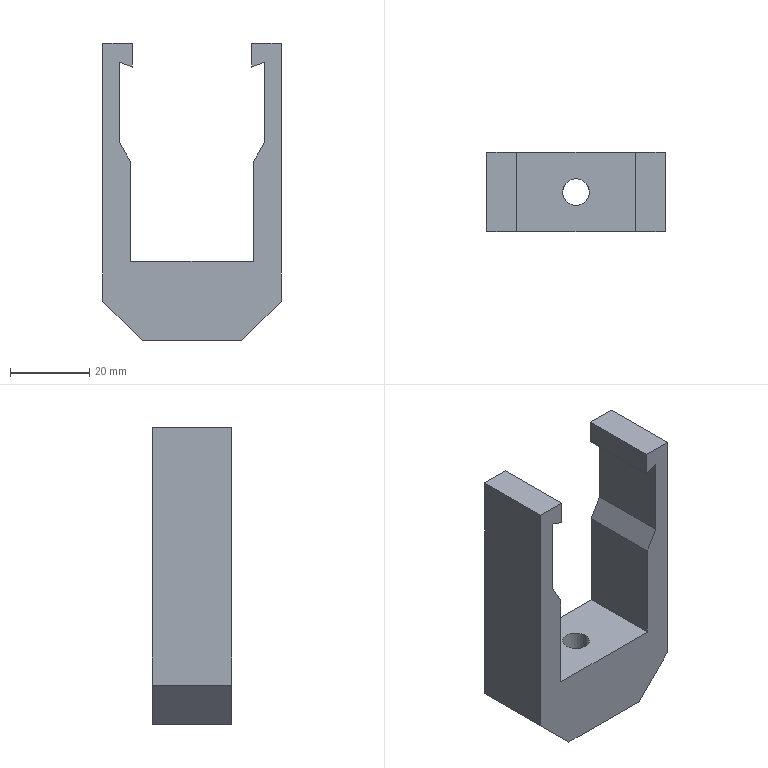Part | STEP file | Blade holder 1 | 1 solid | 22 faces | box 45 x 20 x 75 mm | volume 28350 mm3 | plane 20 | cylinder 2 | commonest cylinder face diameters 6.75 x2
STEP:
#1=CARTESIAN_POINT('',(-3.375,7.5,-37.5));
#2=VERTEX_POINT('',#1);
#3=CARTESIAN_POINT('',(3.375,7.5,-37.5));
#4=VERTEX_POINT('',#3);
#5=CARTESIAN_POINT('',(0.,7.5,-37.5));
#6=DIRECTION('',(0.,0.,1.));
#7=DIRECTION('',(1.,0.,0.));
#8=AXIS2_PLACEMENT_3D('',#5,#6,#7);
#9=CIRCLE('',#8,3.375);
#10=EDGE_CURVE('',#2,#4,#9,.T.);
#11=ORIENTED_EDGE('',*,*,#10,.F.);
#12=CARTESIAN_POINT('',(-3.375,7.5,-17.5));
#13=VERTEX_POINT('',#12);
#14=CARTESIAN_POINT('',(-3.375,7.5,-17.5));
#15=DIRECTION('',(0.,0.,1.));
#16=VECTOR('',#15,1000.);
#17=LINE('',#14,#16);
#18=EDGE_CURVE('',#2,#13,#17,.T.);
#19=ORIENTED_EDGE('',*,*,#18,.T.);
#20=CARTESIAN_POINT('',(3.375,7.5,-17.5));
#21=VERTEX_POINT('',#20);
#22=CARTESIAN_POINT('',(0.,7.5,-17.5));
#23=DIRECTION('',(0.,0.,1.));
#24=DIRECTION('',(1.,0.,0.));
#25=AXIS2_PLACEMENT_3D('',#22,#23,#24);
#26=CIRCLE('',#25,3.375);
#27=EDGE_CURVE('',#13,#21,#26,.T.);
#28=ORIENTED_EDGE('',*,*,#27,.T.);
#29=CARTESIAN_POINT('',(3.375,7.5,-17.5));
#30=DIRECTION('',(0.,0.,1.));
#31=VECTOR('',#30,1000.);
#32=LINE('',#29,#31);
#33=EDGE_CURVE('',#4,#21,#32,.T.);
#34=ORIENTED_EDGE('',*,*,#33,.F.);
#35=EDGE_LOOP('',(#11,#19,#28,#34));
#36=FACE_OUTER_BOUND('',#35,.T.);
#37=CARTESIAN_POINT('',(0.,7.5,-17.5));
#38=DIRECTION('',(0.,0.,1.));
#39=DIRECTION('',(1.,0.,0.));
#40=AXIS2_PLACEMENT_3D('',#37,#38,#39);
#41=CYLINDRICAL_SURFACE('',#40,3.375);
#42=ADVANCED_FACE('',(#36),#41,.F.);
#43=CARTESIAN_POINT('',(15.,17.5,37.5));
#44=VERTEX_POINT('',#43);
#45=CARTESIAN_POINT('',(15.,-2.5,37.5));
#46=VERTEX_POINT('',#45);
#47=CARTESIAN_POINT('',(15.,17.5,37.5));
#48=DIRECTION('',(0.,-1.,0.));
#49=VECTOR('',#48,1000.);
#50=LINE('',#47,#49);
#51=EDGE_CURVE('',#44,#46,#50,.T.);
#52=ORIENTED_EDGE('',*,*,#51,.T.);
#53=CARTESIAN_POINT('',(22.5,-2.5,37.5));
#54=VERTEX_POINT('',#53);
#55=CARTESIAN_POINT('',(-22.5,-2.5,37.5));
#56=DIRECTION('',(1.,0.,0.));
#57=VECTOR('',#56,1000.);
#58=LINE('',#55,#57);
#59=EDGE_CURVE('',#46,#54,#58,.T.);
#60=ORIENTED_EDGE('',*,*,#59,.T.);
#61=CARTESIAN_POINT('',(22.5,17.5,37.5));
#62=VERTEX_POINT('',#61);
#63=CARTESIAN_POINT('',(22.5,-2.5,37.5));
#64=DIRECTION('',(0.,1.,0.));
#65=VECTOR('',#64,1000.);
#66=LINE('',#63,#65);
#67=EDGE_CURVE('',#54,#62,#66,.T.);
#68=ORIENTED_EDGE('',*,*,#67,.T.);
#69=CARTESIAN_POINT('',(-22.5,17.5,37.5));
#70=DIRECTION('',(1.,0.,0.));
#71=VECTOR('',#70,1000.);
#72=LINE('',#69,#71);
#73=EDGE_CURVE('',#44,#62,#72,.T.);
#74=ORIENTED_EDGE('',*,*,#73,.F.);
#75=EDGE_LOOP('',(#52,#60,#68,#74));
#76=FACE_OUTER_BOUND('',#75,.T.);
#77=CARTESIAN_POINT('',(-22.5,-2.5,37.5));
#78=DIRECTION('',(0.,0.,1.));
#79=DIRECTION('',(1.,0.,0.));
#80=AXIS2_PLACEMENT_3D('',#77,#78,#79);
#81=PLANE('',#80);
#82=ADVANCED_FACE('',(#76),#81,.T.);
#83=CARTESIAN_POINT('',(22.5,-2.5,-27.5));
#84=VERTEX_POINT('',#83);
#85=CARTESIAN_POINT('',(22.5,-2.5,37.5));
#86=DIRECTION('',(0.,0.,-1.));
#87=VECTOR('',#86,1000.);
#88=LINE('',#85,#87);
#89=EDGE_CURVE('',#54,#84,#88,.T.);
#90=ORIENTED_EDGE('',*,*,#89,.T.);
#91=CARTESIAN_POINT('',(22.5,17.5,-27.5));
#92=VERTEX_POINT('',#91);
#93=CARTESIAN_POINT('',(22.5,-2.5,-27.5));
#94=DIRECTION('',(0.,1.,0.));
#95=VECTOR('',#94,1000.);
#96=LINE('',#93,#95);
#97=EDGE_CURVE('',#84,#92,#96,.T.);
#98=ORIENTED_EDGE('',*,*,#97,.T.);
#99=CARTESIAN_POINT('',(22.5,17.5,37.5));
#100=DIRECTION('',(0.,0.,-1.));
#101=VECTOR('',#100,1000.);
#102=LINE('',#99,#101);
#103=EDGE_CURVE('',#62,#92,#102,.T.);
#104=ORIENTED_EDGE('',*,*,#103,.F.);
#105=ORIENTED_EDGE('',*,*,#67,.F.);
#106=EDGE_LOOP('',(#90,#98,#104,#105));
#107=FACE_OUTER_BOUND('',#106,.T.);
#108=CARTESIAN_POINT('',(22.5,-2.5,37.5));
#109=DIRECTION('',(1.,0.,0.));
#110=DIRECTION('',(0.,0.,-1.));
#111=AXIS2_PLACEMENT_3D('',#108,#109,#110);
#112=PLANE('',#111);
#113=ADVANCED_FACE('',(#107),#112,.T.);
#114=CARTESIAN_POINT('',(-15.,17.5,37.5));
#115=VERTEX_POINT('',#114);
#116=CARTESIAN_POINT('',(-15.,-2.5,37.5));
#117=VERTEX_POINT('',#116);
#118=CARTESIAN_POINT('',(-15.,17.5,37.5));
#119=DIRECTION('',(0.,-1.,0.));
#120=VECTOR('',#119,1000.);
#121=LINE('',#118,#120);
#122=EDGE_CURVE('',#115,#117,#121,.T.);
#123=ORIENTED_EDGE('',*,*,#122,.F.);
#124=CARTESIAN_POINT('',(-22.5,17.5,37.5));
#125=VERTEX_POINT('',#124);
#126=CARTESIAN_POINT('',(-22.5,17.5,37.5));
#127=DIRECTION('',(1.,0.,0.));
#128=VECTOR('',#127,1000.);
#129=LINE('',#126,#128);
#130=EDGE_CURVE('',#125,#115,#129,.T.);
#131=ORIENTED_EDGE('',*,*,#130,.F.);
#132=CARTESIAN_POINT('',(-22.5,-2.5,37.5));
#133=VERTEX_POINT('',#132);
#134=CARTESIAN_POINT('',(-22.5,-2.5,37.5));
#135=DIRECTION('',(0.,1.,0.));
#136=VECTOR('',#135,1000.);
#137=LINE('',#134,#136);
#138=EDGE_CURVE('',#133,#125,#137,.T.);
#139=ORIENTED_EDGE('',*,*,#138,.F.);
#140=CARTESIAN_POINT('',(-22.5,-2.5,37.5));
#141=DIRECTION('',(1.,0.,0.));
#142=VECTOR('',#141,1000.);
#143=LINE('',#140,#142);
#144=EDGE_CURVE('',#133,#117,#143,.T.);
#145=ORIENTED_EDGE('',*,*,#144,.T.);
#146=EDGE_LOOP('',(#123,#131,#139,#145));
#147=FACE_OUTER_BOUND('',#146,.T.);
#148=CARTESIAN_POINT('',(-22.5,-2.5,37.5));
#149=DIRECTION('',(0.,0.,1.));
#150=DIRECTION('',(1.,0.,0.));
#151=AXIS2_PLACEMENT_3D('',#148,#149,#150);
#152=PLANE('',#151);
#153=ADVANCED_FACE('',(#147),#152,.T.);
#154=CARTESIAN_POINT('',(-22.5,17.5,-27.5));
#155=VERTEX_POINT('',#154);
#156=CARTESIAN_POINT('',(-22.5,17.5,-37.5));
#157=DIRECTION('',(0.,0.,1.));
#158=VECTOR('',#157,1000.);
#159=LINE('',#156,#158);
#160=EDGE_CURVE('',#155,#125,#159,.T.);
#161=ORIENTED_EDGE('',*,*,#160,.F.);
#162=CARTESIAN_POINT('',(-22.5,-2.5,-27.5));
#163=VERTEX_POINT('',#162);
#164=CARTESIAN_POINT('',(-22.5,-2.5,-27.5));
#165=DIRECTION('',(0.,-1.,0.));
#166=VECTOR('',#165,1000.);
#167=LINE('',#164,#166);
#168=EDGE_CURVE('',#155,#163,#167,.T.);
#169=ORIENTED_EDGE('',*,*,#168,.T.);
#170=CARTESIAN_POINT('',(-22.5,-2.5,-37.5));
#171=DIRECTION('',(0.,0.,1.));
#172=VECTOR('',#171,1000.);
#173=LINE('',#170,#172);
#174=EDGE_CURVE('',#163,#133,#173,.T.);
#175=ORIENTED_EDGE('',*,*,#174,.T.);
#176=ORIENTED_EDGE('',*,*,#138,.T.);
#177=EDGE_LOOP('',(#161,#169,#175,#176));
#178=FACE_OUTER_BOUND('',#177,.T.);
#179=CARTESIAN_POINT('',(-22.5,-2.5,-37.5));
#180=DIRECTION('',(-1.,0.,0.));
#181=DIRECTION('',(0.,0.,1.));
#182=AXIS2_PLACEMENT_3D('',#179,#180,#181);
#183=PLANE('',#182);
#184=ADVANCED_FACE('',(#178),#183,.T.);
#185=CARTESIAN_POINT('',(0.,7.5,-37.5));
#186=DIRECTION('',(0.,0.,1.));
#187=DIRECTION('',(1.,0.,0.));
#188=AXIS2_PLACEMENT_3D('',#185,#186,#187);
#189=CIRCLE('',#188,3.375);
#190=EDGE_CURVE('',#4,#2,#189,.T.);
#191=ORIENTED_EDGE('',*,*,#190,.T.);
#192=ORIENTED_EDGE('',*,*,#10,.T.);
#193=EDGE_LOOP('',(#191,#192));
#194=FACE_BOUND('',#193,.T.);
#195=CARTESIAN_POINT('',(12.5,-2.5,-37.5));
#196=VERTEX_POINT('',#195);
#197=CARTESIAN_POINT('',(-12.5,-2.5,-37.5));
#198=VERTEX_POINT('',#197);
#199=CARTESIAN_POINT('',(22.5,-2.5,-37.5));
#200=DIRECTION('',(-1.,0.,0.));
#201=VECTOR('',#200,1000.);
#202=LINE('',#199,#201);
#203=EDGE_CURVE('',#196,#198,#202,.T.);
#204=ORIENTED_EDGE('',*,*,#203,.T.);
#205=CARTESIAN_POINT('',(-12.5,17.5,-37.5));
#206=VERTEX_POINT('',#205);
#207=CARTESIAN_POINT('',(-12.5,-2.5,-37.5));
#208=DIRECTION('',(0.,1.,0.));
#209=VECTOR('',#208,1000.);
#210=LINE('',#207,#209);
#211=EDGE_CURVE('',#198,#206,#210,.T.);
#212=ORIENTED_EDGE('',*,*,#211,.T.);
#213=CARTESIAN_POINT('',(12.5,17.5,-37.5));
#214=VERTEX_POINT('',#213);
#215=CARTESIAN_POINT('',(22.5,17.5,-37.5));
#216=DIRECTION('',(-1.,0.,0.));
#217=VECTOR('',#216,1000.);
#218=LINE('',#215,#217);
#219=EDGE_CURVE('',#214,#206,#218,.T.);
#220=ORIENTED_EDGE('',*,*,#219,.F.);
#221=CARTESIAN_POINT('',(12.5,-2.5,-37.5));
#222=DIRECTION('',(0.,-1.,0.));
#223=VECTOR('',#222,1000.);
#224=LINE('',#221,#223);
#225=EDGE_CURVE('',#214,#196,#224,.T.);
#226=ORIENTED_EDGE('',*,*,#225,.T.);
#227=EDGE_LOOP('',(#204,#212,#220,#226));
#228=FACE_OUTER_BOUND('',#227,.T.);
#229=CARTESIAN_POINT('',(22.5,-2.5,-37.5));
#230=DIRECTION('',(0.,0.,-1.));
#231=DIRECTION('',(-1.,0.,0.));
#232=AXIS2_PLACEMENT_3D('',#229,#230,#231);
#233=PLANE('',#232);
#234=ADVANCED_FACE('',(#194,#228),#233,.T.);
#235=ORIENTED_EDGE('',*,*,#174,.F.);
#236=CARTESIAN_POINT('',(-12.5,-2.5,-37.5));
#237=DIRECTION('',(0.7071,0.,-0.7071));
#238=VECTOR('',#237,1000.);
#239=LINE('',#236,#238);
#240=EDGE_CURVE('',#163,#198,#239,.T.);
#241=ORIENTED_EDGE('',*,*,#240,.T.);
#242=ORIENTED_EDGE('',*,*,#203,.F.);
#243=CARTESIAN_POINT('',(22.5,-2.5,-27.5));
#244=DIRECTION('',(0.7071,0.,0.7071));
#245=VECTOR('',#244,1000.);
#246=LINE('',#243,#245);
#247=EDGE_CURVE('',#196,#84,#246,.T.);
#248=ORIENTED_EDGE('',*,*,#247,.T.);
#249=ORIENTED_EDGE('',*,*,#89,.F.);
#250=ORIENTED_EDGE('',*,*,#59,.F.);
#251=CARTESIAN_POINT('',(15.,-2.5,31.5));
#252=VERTEX_POINT('',#251);
#253=CARTESIAN_POINT('',(15.,-2.5,32.737));
#254=DIRECTION('',(0.,0.,1.));
#255=VECTOR('',#254,1000.);
#256=LINE('',#253,#255);
#257=EDGE_CURVE('',#252,#46,#256,.T.);
#258=ORIENTED_EDGE('',*,*,#257,.F.);
#259=CARTESIAN_POINT('',(18.4,-2.5,32.737));
#260=VERTEX_POINT('',#259);
#261=CARTESIAN_POINT('',(18.4,-2.5,32.737));
#262=DIRECTION('',(-0.9397,0.,-0.342));
#263=VECTOR('',#262,1000.);
#264=LINE('',#261,#263);
#265=EDGE_CURVE('',#260,#252,#264,.T.);
#266=ORIENTED_EDGE('',*,*,#265,.F.);
#267=CARTESIAN_POINT('',(18.4,-2.5,12.737));
#268=VERTEX_POINT('',#267);
#269=CARTESIAN_POINT('',(18.4,-2.5,12.737));
#270=DIRECTION('',(0.,0.,1.));
#271=VECTOR('',#270,1000.);
#272=LINE('',#269,#271);
#273=EDGE_CURVE('',#268,#260,#272,.T.);
#274=ORIENTED_EDGE('',*,*,#273,.F.);
#275=CARTESIAN_POINT('',(15.4,-2.5,7.5));
#276=VERTEX_POINT('',#275);
#277=CARTESIAN_POINT('',(18.4,-2.5,12.737));
#278=DIRECTION('',(0.497,0.,0.8677));
#279=VECTOR('',#278,1000.);
#280=LINE('',#277,#279);
#281=EDGE_CURVE('',#276,#268,#280,.T.);
#282=ORIENTED_EDGE('',*,*,#281,.F.);
#283=CARTESIAN_POINT('',(15.4,-2.5,-17.5));
#284=VERTEX_POINT('',#283);
#285=CARTESIAN_POINT('',(15.4,-2.5,-17.5));
#286=DIRECTION('',(0.,0.,1.));
#287=VECTOR('',#286,1000.);
#288=LINE('',#285,#287);
#289=EDGE_CURVE('',#284,#276,#288,.T.);
#290=ORIENTED_EDGE('',*,*,#289,.F.);
#291=CARTESIAN_POINT('',(-15.4,-2.5,-17.5));
#292=VERTEX_POINT('',#291);
#293=CARTESIAN_POINT('',(-15.4,-2.5,-17.5));
#294=DIRECTION('',(1.,0.,0.));
#295=VECTOR('',#294,1000.);
#296=LINE('',#293,#295);
#297=EDGE_CURVE('',#292,#284,#296,.T.);
#298=ORIENTED_EDGE('',*,*,#297,.F.);
#299=CARTESIAN_POINT('',(-15.4,-2.5,7.5));
#300=VERTEX_POINT('',#299);
#301=CARTESIAN_POINT('',(-15.4,-2.5,7.5));
#302=DIRECTION('',(0.,0.,-1.));
#303=VECTOR('',#302,1000.);
#304=LINE('',#301,#303);
#305=EDGE_CURVE('',#300,#292,#304,.T.);
#306=ORIENTED_EDGE('',*,*,#305,.F.);
#307=CARTESIAN_POINT('',(-18.4,-2.5,12.737));
#308=VERTEX_POINT('',#307);
#309=CARTESIAN_POINT('',(-15.4,-2.5,7.5));
#310=DIRECTION('',(0.497,0.,-0.8677));
#311=VECTOR('',#310,1000.);
#312=LINE('',#309,#311);
#313=EDGE_CURVE('',#308,#300,#312,.T.);
#314=ORIENTED_EDGE('',*,*,#313,.F.);
#315=CARTESIAN_POINT('',(-18.4,-2.5,32.737));
#316=VERTEX_POINT('',#315);
#317=CARTESIAN_POINT('',(-18.4,-2.5,32.737));
#318=DIRECTION('',(0.,0.,-1.));
#319=VECTOR('',#318,1000.);
#320=LINE('',#317,#319);
#321=EDGE_CURVE('',#316,#308,#320,.T.);
#322=ORIENTED_EDGE('',*,*,#321,.F.);
#323=CARTESIAN_POINT('',(-15.,-2.5,31.5));
#324=VERTEX_POINT('',#323);
#325=CARTESIAN_POINT('',(-18.4,-2.5,32.737));
#326=DIRECTION('',(-0.9397,0.,0.342));
#327=VECTOR('',#326,1000.);
#328=LINE('',#325,#327);
#329=EDGE_CURVE('',#324,#316,#328,.T.);
#330=ORIENTED_EDGE('',*,*,#329,.F.);
#331=CARTESIAN_POINT('',(-15.,-2.5,37.5));
#332=DIRECTION('',(0.,0.,-1.));
#333=VECTOR('',#332,1000.);
#334=LINE('',#331,#333);
#335=EDGE_CURVE('',#117,#324,#334,.T.);
#336=ORIENTED_EDGE('',*,*,#335,.F.);
#337=ORIENTED_EDGE('',*,*,#144,.F.);
#338=EDGE_LOOP('',(#235,#241,#242,#248,#249,#250,#258,#266,#274,#282,#290,#298,#306,#314,#322,#330,#336,#337));
#339=FACE_OUTER_BOUND('',#338,.T.);
#340=CARTESIAN_POINT('',(0.,-2.5,0.));
#341=DIRECTION('',(0.,1.,0.));
#342=DIRECTION('',(0.,0.,1.));
#343=AXIS2_PLACEMENT_3D('',#340,#341,#342);
#344=PLANE('',#343);
#345=ADVANCED_FACE('',(#339),#344,.F.);
#346=ORIENTED_EDGE('',*,*,#219,.T.);
#347=CARTESIAN_POINT('',(-25.,17.5,-25.));
#348=DIRECTION('',(-0.7071,0.,0.7071));
#349=VECTOR('',#348,1000.);
#350=LINE('',#347,#349);
#351=EDGE_CURVE('',#206,#155,#350,.T.);
#352=ORIENTED_EDGE('',*,*,#351,.T.);
#353=ORIENTED_EDGE('',*,*,#160,.T.);
#354=ORIENTED_EDGE('',*,*,#130,.T.);
#355=CARTESIAN_POINT('',(-15.,17.5,31.5));
#356=VERTEX_POINT('',#355);
#357=CARTESIAN_POINT('',(-15.,17.5,37.5));
#358=DIRECTION('',(0.,0.,-1.));
#359=VECTOR('',#358,1000.);
#360=LINE('',#357,#359);
#361=EDGE_CURVE('',#115,#356,#360,.T.);
#362=ORIENTED_EDGE('',*,*,#361,.T.);
#363=CARTESIAN_POINT('',(-18.4,17.5,32.737));
#364=VERTEX_POINT('',#363);
#365=CARTESIAN_POINT('',(-18.4,17.5,32.737));
#366=DIRECTION('',(-0.9397,0.,0.342));
#367=VECTOR('',#366,1000.);
#368=LINE('',#365,#367);
#369=EDGE_CURVE('',#356,#364,#368,.T.);
#370=ORIENTED_EDGE('',*,*,#369,.T.);
#371=CARTESIAN_POINT('',(-18.4,17.5,12.737));
#372=VERTEX_POINT('',#371);
#373=CARTESIAN_POINT('',(-18.4,17.5,32.737));
#374=DIRECTION('',(0.,0.,-1.));
#375=VECTOR('',#374,1000.);
#376=LINE('',#373,#375);
#377=EDGE_CURVE('',#364,#372,#376,.T.);
#378=ORIENTED_EDGE('',*,*,#377,.T.);
#379=CARTESIAN_POINT('',(-15.4,17.5,7.5));
#380=VERTEX_POINT('',#379);
#381=CARTESIAN_POINT('',(-15.4,17.5,7.5));
#382=DIRECTION('',(0.497,0.,-0.8677));
#383=VECTOR('',#382,1000.);
#384=LINE('',#381,#383);
#385=EDGE_CURVE('',#372,#380,#384,.T.);
#386=ORIENTED_EDGE('',*,*,#385,.T.);
#387=CARTESIAN_POINT('',(-15.4,17.5,-17.5));
#388=VERTEX_POINT('',#387);
#389=CARTESIAN_POINT('',(-15.4,17.5,7.5));
#390=DIRECTION('',(0.,0.,-1.));
#391=VECTOR('',#390,1000.);
#392=LINE('',#389,#391);
#393=EDGE_CURVE('',#380,#388,#392,.T.);
#394=ORIENTED_EDGE('',*,*,#393,.T.);
#395=CARTESIAN_POINT('',(15.4,17.5,-17.5));
#396=VERTEX_POINT('',#395);
#397=CARTESIAN_POINT('',(-15.4,17.5,-17.5));
#398=DIRECTION('',(1.,0.,0.));
#399=VECTOR('',#398,1000.);
#400=LINE('',#397,#399);
#401=EDGE_CURVE('',#388,#396,#400,.T.);
#402=ORIENTED_EDGE('',*,*,#401,.T.);
#403=CARTESIAN_POINT('',(15.4,17.5,7.5));
#404=VERTEX_POINT('',#403);
#405=CARTESIAN_POINT('',(15.4,17.5,-17.5));
#406=DIRECTION('',(0.,0.,1.));
#407=VECTOR('',#406,1000.);
#408=LINE('',#405,#407);
#409=EDGE_CURVE('',#396,#404,#408,.T.);
#410=ORIENTED_EDGE('',*,*,#409,.T.);
#411=CARTESIAN_POINT('',(18.4,17.5,12.737));
#412=VERTEX_POINT('',#411);
#413=CARTESIAN_POINT('',(18.4,17.5,12.737));
#414=DIRECTION('',(0.497,0.,0.8677));
#415=VECTOR('',#414,1000.);
#416=LINE('',#413,#415);
#417=EDGE_CURVE('',#404,#412,#416,.T.);
#418=ORIENTED_EDGE('',*,*,#417,.T.);
#419=CARTESIAN_POINT('',(18.4,17.5,32.737));
#420=VERTEX_POINT('',#419);
#421=CARTESIAN_POINT('',(18.4,17.5,12.737));
#422=DIRECTION('',(0.,0.,1.));
#423=VECTOR('',#422,1000.);
#424=LINE('',#421,#423);
#425=EDGE_CURVE('',#412,#420,#424,.T.);
#426=ORIENTED_EDGE('',*,*,#425,.T.);
#427=CARTESIAN_POINT('',(15.,17.5,31.5));
#428=VERTEX_POINT('',#427);
#429=CARTESIAN_POINT('',(18.4,17.5,32.737));
#430=DIRECTION('',(-0.9397,0.,-0.342));
#431=VECTOR('',#430,1000.);
#432=LINE('',#429,#431);
#433=EDGE_CURVE('',#420,#428,#432,.T.);
#434=ORIENTED_EDGE('',*,*,#433,.T.);
#435=CARTESIAN_POINT('',(15.,17.5,32.737));
#436=DIRECTION('',(0.,0.,1.));
#437=VECTOR('',#436,1000.);
#438=LINE('',#435,#437);
#439=EDGE_CURVE('',#428,#44,#438,.T.);
#440=ORIENTED_EDGE('',*,*,#439,.T.);
#441=ORIENTED_EDGE('',*,*,#73,.T.);
#442=ORIENTED_EDGE('',*,*,#103,.T.);
#443=CARTESIAN_POINT('',(25.,17.5,-25.));
#444=DIRECTION('',(-0.7071,0.,-0.7071));
#445=VECTOR('',#444,1000.);
#446=LINE('',#443,#445);
#447=EDGE_CURVE('',#92,#214,#446,.T.);
#448=ORIENTED_EDGE('',*,*,#447,.T.);
#449=EDGE_LOOP('',(#346,#352,#353,#354,#362,#370,#378,#386,#394,#402,#410,#418,#426,#434,#440,#441,#442,#448));
#450=FACE_OUTER_BOUND('',#449,.T.);
#451=CARTESIAN_POINT('',(0.,17.5,0.));
#452=DIRECTION('',(0.,1.,0.));
#453=DIRECTION('',(0.,0.,1.));
#454=AXIS2_PLACEMENT_3D('',#451,#452,#453);
#455=PLANE('',#454);
#456=ADVANCED_FACE('',(#450),#455,.T.);
#457=ORIENTED_EDGE('',*,*,#257,.T.);
#458=ORIENTED_EDGE('',*,*,#51,.F.);
#459=ORIENTED_EDGE('',*,*,#439,.F.);
#460=CARTESIAN_POINT('',(15.,17.5,31.5));
#461=DIRECTION('',(0.,-1.,0.));
#462=VECTOR('',#461,1000.);
#463=LINE('',#460,#462);
#464=EDGE_CURVE('',#428,#252,#463,.T.);
#465=ORIENTED_EDGE('',*,*,#464,.T.);
#466=EDGE_LOOP('',(#457,#458,#459,#465));
#467=FACE_OUTER_BOUND('',#466,.T.);
#468=CARTESIAN_POINT('',(15.,17.5,32.737));
#469=DIRECTION('',(1.,0.,0.));
#470=DIRECTION('',(0.,0.,-1.));
#471=AXIS2_PLACEMENT_3D('',#468,#469,#470);
#472=PLANE('',#471);
#473=ADVANCED_FACE('',(#467),#472,.F.);
#474=ORIENTED_EDGE('',*,*,#265,.T.);
#475=ORIENTED_EDGE('',*,*,#464,.F.);
#476=ORIENTED_EDGE('',*,*,#433,.F.);
#477=CARTESIAN_POINT('',(18.4,17.5,32.737));
#478=DIRECTION('',(0.,-1.,0.));
#479=VECTOR('',#478,1000.);
#480=LINE('',#477,#479);
#481=EDGE_CURVE('',#420,#260,#480,.T.);
#482=ORIENTED_EDGE('',*,*,#481,.T.);
#483=EDGE_LOOP('',(#474,#475,#476,#482));
#484=FACE_OUTER_BOUND('',#483,.T.);
#485=CARTESIAN_POINT('',(18.4,17.5,32.737));
#486=DIRECTION('',(0.342,0.,-0.9397));
#487=DIRECTION('',(-0.9397,0.,-0.342));
#488=AXIS2_PLACEMENT_3D('',#485,#486,#487);
#489=PLANE('',#488);
#490=ADVANCED_FACE('',(#484),#489,.T.);
#491=ORIENTED_EDGE('',*,*,#273,.T.);
#492=ORIENTED_EDGE('',*,*,#481,.F.);
#493=ORIENTED_EDGE('',*,*,#425,.F.);
#494=CARTESIAN_POINT('',(18.4,17.5,12.737));
#495=DIRECTION('',(0.,-1.,0.));
#496=VECTOR('',#495,1000.);
#497=LINE('',#494,#496);
#498=EDGE_CURVE('',#412,#268,#497,.T.);
#499=ORIENTED_EDGE('',*,*,#498,.T.);
#500=EDGE_LOOP('',(#491,#492,#493,#499));
#501=FACE_OUTER_BOUND('',#500,.T.);
#502=CARTESIAN_POINT('',(18.4,17.5,12.737));
#503=DIRECTION('',(1.,0.,0.));
#504=DIRECTION('',(0.,0.,-1.));
#505=AXIS2_PLACEMENT_3D('',#502,#503,#504);
#506=PLANE('',#505);
#507=ADVANCED_FACE('',(#501),#506,.F.);
#508=ORIENTED_EDGE('',*,*,#281,.T.);
#509=ORIENTED_EDGE('',*,*,#498,.F.);
#510=ORIENTED_EDGE('',*,*,#417,.F.);
#511=CARTESIAN_POINT('',(15.4,17.5,7.5));
#512=DIRECTION('',(0.,-1.,0.));
#513=VECTOR('',#512,1000.);
#514=LINE('',#511,#513);
#515=EDGE_CURVE('',#404,#276,#514,.T.);
#516=ORIENTED_EDGE('',*,*,#515,.T.);
#517=EDGE_LOOP('',(#508,#509,#510,#516));
#518=FACE_OUTER_BOUND('',#517,.T.);
#519=CARTESIAN_POINT('',(18.4,17.5,12.737));
#520=DIRECTION('',(-0.8677,0.,0.497));
#521=DIRECTION('',(0.497,0.,0.8677));
#522=AXIS2_PLACEMENT_3D('',#519,#520,#521);
#523=PLANE('',#522);
#524=ADVANCED_FACE('',(#518),#523,.T.);
#525=ORIENTED_EDGE('',*,*,#289,.T.);
#526=ORIENTED_EDGE('',*,*,#515,.F.);
#527=ORIENTED_EDGE('',*,*,#409,.F.);
#528=CARTESIAN_POINT('',(15.4,17.5,-17.5));
#529=DIRECTION('',(0.,-1.,0.));
#530=VECTOR('',#529,1000.);
#531=LINE('',#528,#530);
#532=EDGE_CURVE('',#396,#284,#531,.T.);
#533=ORIENTED_EDGE('',*,*,#532,.T.);
#534=EDGE_LOOP('',(#525,#526,#527,#533));
#535=FACE_OUTER_BOUND('',#534,.T.);
#536=CARTESIAN_POINT('',(15.4,17.5,-17.5));
#537=DIRECTION('',(1.,0.,0.));
#538=DIRECTION('',(0.,0.,-1.));
#539=AXIS2_PLACEMENT_3D('',#536,#537,#538);
#540=PLANE('',#539);
#541=ADVANCED_FACE('',(#535),#540,.F.);
#542=CARTESIAN_POINT('',(0.,7.5,-17.5));
#543=DIRECTION('',(0.,0.,1.));
#544=DIRECTION('',(1.,0.,0.));
#545=AXIS2_PLACEMENT_3D('',#542,#543,#544);
#546=CIRCLE('',#545,3.375);
#547=EDGE_CURVE('',#21,#13,#546,.T.);
#548=ORIENTED_EDGE('',*,*,#547,.F.);
#549=ORIENTED_EDGE('',*,*,#27,.F.);
#550=EDGE_LOOP('',(#548,#549));
#551=FACE_BOUND('',#550,.T.);
#552=ORIENTED_EDGE('',*,*,#297,.T.);
#553=ORIENTED_EDGE('',*,*,#532,.F.);
#554=ORIENTED_EDGE('',*,*,#401,.F.);
#555=CARTESIAN_POINT('',(-15.4,17.5,-17.5));
#556=DIRECTION('',(0.,-1.,0.));
#557=VECTOR('',#556,1000.);
#558=LINE('',#555,#557);
#559=EDGE_CURVE('',#388,#292,#558,.T.);
#560=ORIENTED_EDGE('',*,*,#559,.T.);
#561=EDGE_LOOP('',(#552,#553,#554,#560));
#562=FACE_OUTER_BOUND('',#561,.T.);
#563=CARTESIAN_POINT('',(-15.4,17.5,-17.5));
#564=DIRECTION('',(0.,0.,-1.));
#565=DIRECTION('',(0.,1.,0.));
#566=AXIS2_PLACEMENT_3D('',#563,#564,#565);
#567=PLANE('',#566);
#568=ADVANCED_FACE('',(#551,#562),#567,.F.);
#569=ORIENTED_EDGE('',*,*,#305,.T.);
#570=ORIENTED_EDGE('',*,*,#559,.F.);
#571=ORIENTED_EDGE('',*,*,#393,.F.);
#572=CARTESIAN_POINT('',(-15.4,17.5,7.5));
#573=DIRECTION('',(0.,-1.,0.));
#574=VECTOR('',#573,1000.);
#575=LINE('',#572,#574);
#576=EDGE_CURVE('',#380,#300,#575,.T.);
#577=ORIENTED_EDGE('',*,*,#576,.T.);
#578=EDGE_LOOP('',(#569,#570,#571,#577));
#579=FACE_OUTER_BOUND('',#578,.T.);
#580=CARTESIAN_POINT('',(-15.4,17.5,7.5));
#581=DIRECTION('',(-1.,0.,0.));
#582=DIRECTION('',(0.,0.,1.));
#583=AXIS2_PLACEMENT_3D('',#580,#581,#582);
#584=PLANE('',#583);
#585=ADVANCED_FACE('',(#579),#584,.F.);
#586=ORIENTED_EDGE('',*,*,#313,.T.);
#587=ORIENTED_EDGE('',*,*,#576,.F.);
#588=ORIENTED_EDGE('',*,*,#385,.F.);
#589=CARTESIAN_POINT('',(-18.4,17.5,12.737));
#590=DIRECTION('',(0.,-1.,0.));
#591=VECTOR('',#590,1000.);
#592=LINE('',#589,#591);
#593=EDGE_CURVE('',#372,#308,#592,.T.);
#594=ORIENTED_EDGE('',*,*,#593,.T.);
#595=EDGE_LOOP('',(#586,#587,#588,#594));
#596=FACE_OUTER_BOUND('',#595,.T.);
#597=CARTESIAN_POINT('',(-15.4,17.5,7.5));
#598=DIRECTION('',(0.8677,0.,0.497));
#599=DIRECTION('',(0.497,0.,-0.8677));
#600=AXIS2_PLACEMENT_3D('',#597,#598,#599);
#601=PLANE('',#600);
#602=ADVANCED_FACE('',(#596),#601,.T.);
#603=ORIENTED_EDGE('',*,*,#321,.T.);
#604=ORIENTED_EDGE('',*,*,#593,.F.);
#605=ORIENTED_EDGE('',*,*,#377,.F.);
#606=CARTESIAN_POINT('',(-18.4,17.5,32.737));
#607=DIRECTION('',(0.,-1.,0.));
#608=VECTOR('',#607,1000.);
#609=LINE('',#606,#608);
#610=EDGE_CURVE('',#364,#316,#609,.T.);
#611=ORIENTED_EDGE('',*,*,#610,.T.);
#612=EDGE_LOOP('',(#603,#604,#605,#611));
#613=FACE_OUTER_BOUND('',#612,.T.);
#614=CARTESIAN_POINT('',(-18.4,17.5,32.737));
#615=DIRECTION('',(-1.,0.,0.));
#616=DIRECTION('',(0.,0.,1.));
#617=AXIS2_PLACEMENT_3D('',#614,#615,#616);
#618=PLANE('',#617);
#619=ADVANCED_FACE('',(#613),#618,.F.);
#620=ORIENTED_EDGE('',*,*,#329,.T.);
#621=ORIENTED_EDGE('',*,*,#610,.F.);
#622=ORIENTED_EDGE('',*,*,#369,.F.);
#623=CARTESIAN_POINT('',(-15.,17.5,31.5));
#624=DIRECTION('',(0.,-1.,0.));
#625=VECTOR('',#624,1000.);
#626=LINE('',#623,#625);
#627=EDGE_CURVE('',#356,#324,#626,.T.);
#628=ORIENTED_EDGE('',*,*,#627,.T.);
#629=EDGE_LOOP('',(#620,#621,#622,#628));
#630=FACE_OUTER_BOUND('',#629,.T.);
#631=CARTESIAN_POINT('',(-18.4,17.5,32.737));
#632=DIRECTION('',(-0.342,0.,-0.9397));
#633=DIRECTION('',(-0.9397,0.,0.342));
#634=AXIS2_PLACEMENT_3D('',#631,#632,#633);
#635=PLANE('',#634);
#636=ADVANCED_FACE('',(#630),#635,.T.);
#637=ORIENTED_EDGE('',*,*,#335,.T.);
#638=ORIENTED_EDGE('',*,*,#627,.F.);
#639=ORIENTED_EDGE('',*,*,#361,.F.);
#640=ORIENTED_EDGE('',*,*,#122,.T.);
#641=EDGE_LOOP('',(#637,#638,#639,#640));
#642=FACE_OUTER_BOUND('',#641,.T.);
#643=CARTESIAN_POINT('',(-15.,17.5,37.5));
#644=DIRECTION('',(-1.,0.,0.));
#645=DIRECTION('',(0.,0.,1.));
#646=AXIS2_PLACEMENT_3D('',#643,#644,#645);
#647=PLANE('',#646);
#648=ADVANCED_FACE('',(#642),#647,.F.);
#649=ORIENTED_EDGE('',*,*,#18,.F.);
#650=ORIENTED_EDGE('',*,*,#190,.F.);
#651=ORIENTED_EDGE('',*,*,#33,.T.);
#652=ORIENTED_EDGE('',*,*,#547,.T.);
#653=EDGE_LOOP('',(#649,#650,#651,#652));
#654=FACE_OUTER_BOUND('',#653,.T.);
#655=CARTESIAN_POINT('',(0.,7.5,-17.5));
#656=DIRECTION('',(0.,0.,1.));
#657=DIRECTION('',(1.,0.,0.));
#658=AXIS2_PLACEMENT_3D('',#655,#656,#657);
#659=CYLINDRICAL_SURFACE('',#658,3.375);
#660=ADVANCED_FACE('',(#654),#659,.F.);
#661=ORIENTED_EDGE('',*,*,#240,.F.);
#662=ORIENTED_EDGE('',*,*,#168,.F.);
#663=ORIENTED_EDGE('',*,*,#351,.F.);
#664=ORIENTED_EDGE('',*,*,#211,.F.);
#665=EDGE_LOOP('',(#661,#662,#663,#664));
#666=FACE_OUTER_BOUND('',#665,.T.);
#667=CARTESIAN_POINT('',(-12.5,-2.5,-37.5));
#668=DIRECTION('',(0.7071,0.,0.7071));
#669=DIRECTION('',(0.,1.,0.));
#670=AXIS2_PLACEMENT_3D('',#667,#668,#669);
#671=PLANE('',#670);
#672=ADVANCED_FACE('',(#666),#671,.F.);
#673=ORIENTED_EDGE('',*,*,#247,.F.);
#674=ORIENTED_EDGE('',*,*,#225,.F.);
#675=ORIENTED_EDGE('',*,*,#447,.F.);
#676=ORIENTED_EDGE('',*,*,#97,.F.);
#677=EDGE_LOOP('',(#673,#674,#675,#676));
#678=FACE_OUTER_BOUND('',#677,.T.);
#679=CARTESIAN_POINT('',(22.5,-2.5,-27.5));
#680=DIRECTION('',(-0.7071,0.,0.7071));
#681=DIRECTION('',(0.,1.,0.));
#682=AXIS2_PLACEMENT_3D('',#679,#680,#681);
#683=PLANE('',#682);
#684=ADVANCED_FACE('',(#678),#683,.F.);
#685=CLOSED_SHELL('',(#42,#82,#113,#153,#184,#234,#345,#456,#473,#490,#507,#524,#541,#568,#585,#602,#619,#636,#648,#660,#672,#684));
#686=MANIFOLD_SOLID_BREP('',#685);
#687=CARTESIAN_POINT('',(0.,0.,0.));
#688=DIRECTION('',(0.,0.,1.));
#689=DIRECTION('',(1.,0.,0.));
#690=AXIS2_PLACEMENT_3D('',#687,#688,#689);
#691=(LENGTH_UNIT()NAMED_UNIT(*)SI_UNIT(.MILLI.,.METRE.));
#692=UNCERTAINTY_MEASURE_WITH_UNIT(LENGTH_MEASURE(0.00001),#691,'','');
#693=(NAMED_UNIT(*)PLANE_ANGLE_UNIT()SI_UNIT($,.RADIAN.));
#694=(NAMED_UNIT(*)SI_UNIT($,.STERADIAN.)SOLID_ANGLE_UNIT());
#695=(GEOMETRIC_REPRESENTATION_CONTEXT(3)GLOBAL_UNCERTAINTY_ASSIGNED_CONTEXT((#692))GLOBAL_UNIT_ASSIGNED_CONTEXT((#691,#693,#694))REPRESENTATION_CONTEXT('',''));
#696=ADVANCED_BREP_SHAPE_REPRESENTATION('',(#686,#690),#695);